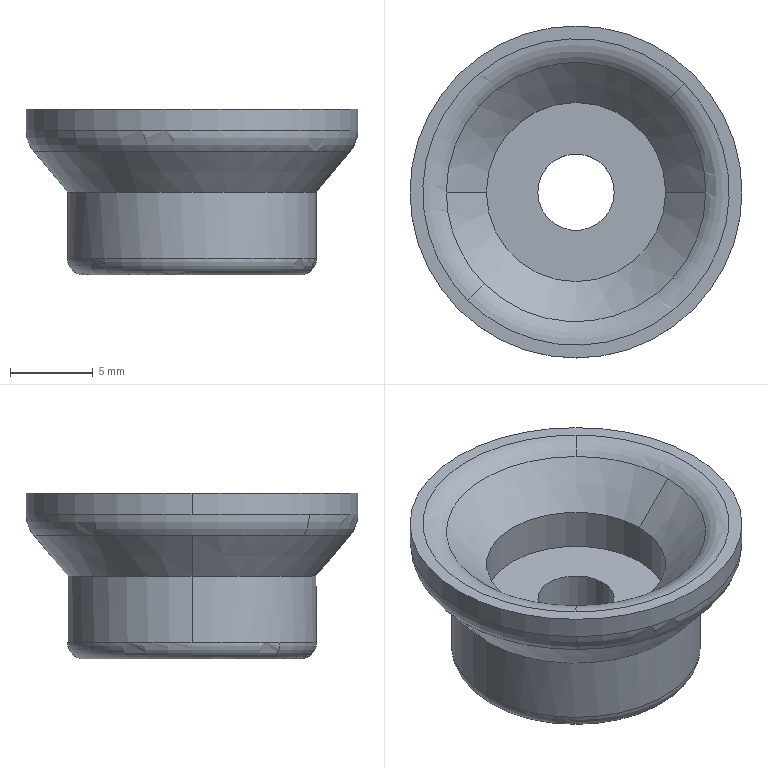Part | STEP file | ASND-0110-Body 1-3 | 1 solid | 21 faces | box 20 x 20 x 10 mm | volume 1461 mm3 | cylinder 8 | torus 6 | cone 4 | plane 3 | commonest cylinder face diameters 4.6 x2 10.8 x2 15 x2 20 x2